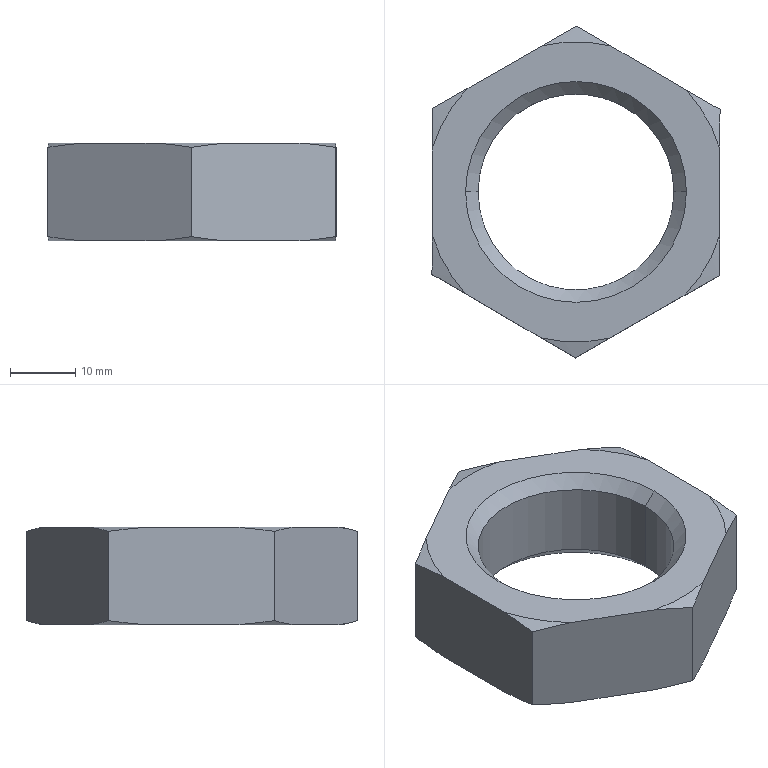Part | STEP file | GB/T6172.1-2000 hex thin nut grade A and B M30 | 1 solid | 26 faces | box 44.137 x 50.85 x 15 mm | volume 14200 mm3 | cone 16 | plane 8 | cylinder 2 | commonest cylinder face diameters 30 x2
STEP:
#1=CARTESIAN_POINT('',(-15.,0.,13.086));
#2=VERTEX_POINT('',#1);
#3=CARTESIAN_POINT('',(15.,0.,13.086));
#4=VERTEX_POINT('',#3);
#5=CARTESIAN_POINT('',(0.,0.,13.086));
#6=DIRECTION('',(0.,0.,1.));
#7=DIRECTION('',(1.,0.,0.));
#8=AXIS2_PLACEMENT_3D('',#5,#6,#7);
#9=CIRCLE('',#8,15.);
#10=EDGE_CURVE('',#2,#4,#9,.T.);
#11=ORIENTED_EDGE('',*,*,#10,.F.);
#12=CARTESIAN_POINT('',(-16.914,0.,15.));
#13=VERTEX_POINT('',#12);
#14=CARTESIAN_POINT('',(-15.,0.,13.086));
#15=DIRECTION('',(-0.7071,0.,0.7071));
#16=VECTOR('',#15,1000.);
#17=LINE('',#14,#16);
#18=EDGE_CURVE('',#2,#13,#17,.T.);
#19=ORIENTED_EDGE('',*,*,#18,.T.);
#20=CARTESIAN_POINT('',(16.914,0.,15.));
#21=VERTEX_POINT('',#20);
#22=CARTESIAN_POINT('',(0.,0.,15.));
#23=DIRECTION('',(0.,0.,-1.));
#24=DIRECTION('',(1.,0.,0.));
#25=AXIS2_PLACEMENT_3D('',#22,#23,#24);
#26=CIRCLE('',#25,16.914);
#27=EDGE_CURVE('',#21,#13,#26,.T.);
#28=ORIENTED_EDGE('',*,*,#27,.F.);
#29=CARTESIAN_POINT('',(15.,0.,13.086));
#30=DIRECTION('',(0.7071,0.,0.7071));
#31=VECTOR('',#30,1000.);
#32=LINE('',#29,#31);
#33=EDGE_CURVE('',#4,#21,#32,.T.);
#34=ORIENTED_EDGE('',*,*,#33,.F.);
#35=EDGE_LOOP('',(#11,#19,#28,#34));
#36=FACE_OUTER_BOUND('',#35,.T.);
#37=CARTESIAN_POINT('',(0.,0.,13.086));
#38=DIRECTION('',(0.,0.,1.));
#39=DIRECTION('',(1.,0.,0.));
#40=AXIS2_PLACEMENT_3D('',#37,#38,#39);
#41=CONICAL_SURFACE('',#40,15.,0.7854);
#42=ADVANCED_FACE('',(#36),#41,.F.);
#43=CARTESIAN_POINT('',(15.,0.,1.914));
#44=VERTEX_POINT('',#43);
#45=CARTESIAN_POINT('',(-15.,0.,1.914));
#46=VERTEX_POINT('',#45);
#47=CARTESIAN_POINT('',(0.,0.,1.914));
#48=DIRECTION('',(0.,0.,-1.));
#49=DIRECTION('',(1.,0.,0.));
#50=AXIS2_PLACEMENT_3D('',#47,#48,#49);
#51=CIRCLE('',#50,15.);
#52=EDGE_CURVE('',#44,#46,#51,.T.);
#53=ORIENTED_EDGE('',*,*,#52,.F.);
#54=CARTESIAN_POINT('',(16.914,0.,0.));
#55=VERTEX_POINT('',#54);
#56=CARTESIAN_POINT('',(16.914,0.,0.));
#57=DIRECTION('',(0.7071,0.,-0.7071));
#58=VECTOR('',#57,1000.);
#59=LINE('',#56,#58);
#60=EDGE_CURVE('',#44,#55,#59,.T.);
#61=ORIENTED_EDGE('',*,*,#60,.T.);
#62=CARTESIAN_POINT('',(-16.914,0.,0.));
#63=VERTEX_POINT('',#62);
#64=CARTESIAN_POINT('',(0.,0.,0.));
#65=DIRECTION('',(0.,0.,1.));
#66=DIRECTION('',(1.,0.,0.));
#67=AXIS2_PLACEMENT_3D('',#64,#65,#66);
#68=CIRCLE('',#67,16.914);
#69=EDGE_CURVE('',#63,#55,#68,.T.);
#70=ORIENTED_EDGE('',*,*,#69,.F.);
#71=CARTESIAN_POINT('',(-16.914,0.,0.));
#72=DIRECTION('',(-0.7071,0.,-0.7071));
#73=VECTOR('',#72,1000.);
#74=LINE('',#71,#73);
#75=EDGE_CURVE('',#46,#63,#74,.T.);
#76=ORIENTED_EDGE('',*,*,#75,.F.);
#77=EDGE_LOOP('',(#53,#61,#70,#76));
#78=FACE_OUTER_BOUND('',#77,.T.);
#79=CARTESIAN_POINT('',(0.,0.,0.));
#80=DIRECTION('',(0.,0.,-1.));
#81=DIRECTION('',(-1.,0.,0.));
#82=AXIS2_PLACEMENT_3D('',#79,#80,#81);
#83=CONICAL_SURFACE('',#82,16.914,0.7854);
#84=ADVANCED_FACE('',(#78),#83,.F.);
#85=ORIENTED_EDGE('',*,*,#10,.T.);
#86=CARTESIAN_POINT('',(15.,0.,15.));
#87=DIRECTION('',(0.,0.,-1.));
#88=VECTOR('',#87,1000.);
#89=LINE('',#86,#88);
#90=EDGE_CURVE('',#4,#44,#89,.T.);
#91=ORIENTED_EDGE('',*,*,#90,.T.);
#92=ORIENTED_EDGE('',*,*,#52,.T.);
#93=CARTESIAN_POINT('',(-15.,0.,15.));
#94=DIRECTION('',(0.,0.,-1.));
#95=VECTOR('',#94,1000.);
#96=LINE('',#93,#95);
#97=EDGE_CURVE('',#2,#46,#96,.T.);
#98=ORIENTED_EDGE('',*,*,#97,.F.);
#99=EDGE_LOOP('',(#85,#91,#92,#98));
#100=FACE_OUTER_BOUND('',#99,.T.);
#101=CARTESIAN_POINT('',(0.,0.,15.));
#102=DIRECTION('',(0.,0.,-1.));
#103=DIRECTION('',(-1.,0.,0.));
#104=AXIS2_PLACEMENT_3D('',#101,#102,#103);
#105=CYLINDRICAL_SURFACE('',#104,15.);
#106=ADVANCED_FACE('',(#100),#105,.F.);
#107=CARTESIAN_POINT('',(22.069,12.626,14.35));
#108=VERTEX_POINT('',#107);
#109=CARTESIAN_POINT('',(16.827,15.679,15.));
#110=VERTEX_POINT('',#109);
#111=CARTESIAN_POINT('',(22.069,12.626,14.35));
#112=CARTESIAN_POINT('',(20.327,13.641,14.62));
#113=CARTESIAN_POINT('',(18.58,14.658,14.843));
#114=CARTESIAN_POINT('',(16.827,15.679,15.));
#115=B_SPLINE_CURVE_WITH_KNOTS('',3,(#111,#112,#113,#114),.UNSPECIFIED.,.F.,.F.,(4,4),(0.0208,0.0269),.UNSPECIFIED.);
#116=EDGE_CURVE('',#108,#110,#115,.T.);
#117=ORIENTED_EDGE('',*,*,#116,.F.);
#118=CARTESIAN_POINT('',(22.069,12.626,0.6498));
#119=VERTEX_POINT('',#118);
#120=CARTESIAN_POINT('',(22.069,12.626,15.));
#121=DIRECTION('',(0.,0.,-1.));
#122=VECTOR('',#121,1000.);
#123=LINE('',#120,#122);
#124=EDGE_CURVE('',#108,#119,#123,.T.);
#125=ORIENTED_EDGE('',*,*,#124,.T.);
#126=CARTESIAN_POINT('',(16.827,15.679,0.));
#127=VERTEX_POINT('',#126);
#128=CARTESIAN_POINT('',(16.827,15.679,0.));
#129=CARTESIAN_POINT('',(17.704,15.169,0.07853));
#130=CARTESIAN_POINT('',(18.58,14.658,0.1736));
#131=CARTESIAN_POINT('',(20.327,13.64,0.3918));
#132=CARTESIAN_POINT('',(21.199,13.132,0.5149));
#133=CARTESIAN_POINT('',(22.069,12.626,0.6498));
#134=B_SPLINE_CURVE_WITH_KNOTS('',3,(#128,#129,#130,#131,#132,#133),.UNSPECIFIED.,.F.,.F.,(4,2,4),(0.04011,0.04311,0.04611),.UNSPECIFIED.);
#135=EDGE_CURVE('',#127,#119,#134,.T.);
#136=ORIENTED_EDGE('',*,*,#135,.F.);
#137=CARTESIAN_POINT('',(5.341,22.371,0.));
#138=VERTEX_POINT('',#137);
#139=CARTESIAN_POINT('',(22.069,12.626,0.));
#140=DIRECTION('',(-0.8641,0.5034,0.));
#141=VECTOR('',#140,1000.);
#142=LINE('',#139,#141);
#143=EDGE_CURVE('',#127,#138,#142,.T.);
#144=ORIENTED_EDGE('',*,*,#143,.T.);
#145=CARTESIAN_POINT('',(0.1,25.425,0.6498));
#146=VERTEX_POINT('',#145);
#147=CARTESIAN_POINT('',(0.1,25.425,0.6498));
#148=CARTESIAN_POINT('',(1.842,24.41,0.3797));
#149=CARTESIAN_POINT('',(3.589,23.392,0.1571));
#150=CARTESIAN_POINT('',(5.341,22.371,0.));
#151=B_SPLINE_CURVE_WITH_KNOTS('',3,(#147,#148,#149,#150),.UNSPECIFIED.,.F.,.F.,(4,4),(0.0208,0.0269),.UNSPECIFIED.);
#152=EDGE_CURVE('',#146,#138,#151,.T.);
#153=ORIENTED_EDGE('',*,*,#152,.F.);
#154=CARTESIAN_POINT('',(0.1,25.425,14.35));
#155=VERTEX_POINT('',#154);
#156=CARTESIAN_POINT('',(0.1,25.425,15.));
#157=DIRECTION('',(0.,0.,-1.));
#158=VECTOR('',#157,1000.);
#159=LINE('',#156,#158);
#160=EDGE_CURVE('',#155,#146,#159,.T.);
#161=ORIENTED_EDGE('',*,*,#160,.F.);
#162=CARTESIAN_POINT('',(5.341,22.371,15.));
#163=VERTEX_POINT('',#162);
#164=CARTESIAN_POINT('',(5.341,22.371,15.));
#165=CARTESIAN_POINT('',(4.465,22.882,14.921));
#166=CARTESIAN_POINT('',(3.588,23.393,14.826));
#167=CARTESIAN_POINT('',(1.841,24.41,14.608));
#168=CARTESIAN_POINT('',(0.9697,24.918,14.485));
#169=CARTESIAN_POINT('',(0.1,25.425,14.35));
#170=B_SPLINE_CURVE_WITH_KNOTS('',3,(#164,#165,#166,#167,#168,#169),.UNSPECIFIED.,.F.,.F.,(4,2,4),(0.04011,0.04311,0.04611),.UNSPECIFIED.);
#171=EDGE_CURVE('',#163,#155,#170,.T.);
#172=ORIENTED_EDGE('',*,*,#171,.F.);
#173=CARTESIAN_POINT('',(22.069,12.626,15.));
#174=DIRECTION('',(-0.8641,0.5034,0.));
#175=VECTOR('',#174,1000.);
#176=LINE('',#173,#175);
#177=EDGE_CURVE('',#110,#163,#176,.T.);
#178=ORIENTED_EDGE('',*,*,#177,.F.);
#179=EDGE_LOOP('',(#117,#125,#136,#144,#153,#161,#172,#178));
#180=FACE_OUTER_BOUND('',#179,.T.);
#181=CARTESIAN_POINT('',(22.069,12.626,15.));
#182=DIRECTION('',(-0.5034,-0.8641,0.));
#183=DIRECTION('',(0.8641,-0.5034,0.));
#184=AXIS2_PLACEMENT_3D('',#181,#182,#183);
#185=PLANE('',#184);
#186=ADVANCED_FACE('',(#180),#185,.F.);
#187=CARTESIAN_POINT('',(-5.165,22.413,15.));
#188=VERTEX_POINT('',#187);
#189=CARTESIAN_POINT('',(0.1,25.425,14.35));
#190=CARTESIAN_POINT('',(-1.65,24.424,14.62));
#191=CARTESIAN_POINT('',(-3.404,23.42,14.843));
#192=CARTESIAN_POINT('',(-5.165,22.413,15.));
#193=B_SPLINE_CURVE_WITH_KNOTS('',3,(#189,#190,#191,#192),.UNSPECIFIED.,.F.,.F.,(4,4),(0.0207,0.0268),.UNSPECIFIED.);
#194=EDGE_CURVE('',#155,#188,#193,.T.);
#195=ORIENTED_EDGE('',*,*,#194,.F.);
#196=ORIENTED_EDGE('',*,*,#160,.T.);
#197=CARTESIAN_POINT('',(-5.165,22.413,0.));
#198=VERTEX_POINT('',#197);
#199=CARTESIAN_POINT('',(-5.165,22.413,0.));
#200=CARTESIAN_POINT('',(-4.285,22.916,0.07852));
#201=CARTESIAN_POINT('',(-3.404,23.42,0.1736));
#202=CARTESIAN_POINT('',(-1.649,24.424,0.3918));
#203=CARTESIAN_POINT('',(-0.7736,24.925,0.5149));
#204=CARTESIAN_POINT('',(0.1,25.425,0.6498));
#205=B_SPLINE_CURVE_WITH_KNOTS('',3,(#199,#200,#201,#202,#203,#204),.UNSPECIFIED.,.F.,.F.,(4,2,4),(0.04002,0.04302,0.04602),.UNSPECIFIED.);
#206=EDGE_CURVE('',#198,#146,#205,.T.);
#207=ORIENTED_EDGE('',*,*,#206,.F.);
#208=CARTESIAN_POINT('',(-16.703,15.811,0.));
#209=VERTEX_POINT('',#208);
#210=CARTESIAN_POINT('',(0.1,25.425,0.));
#211=DIRECTION('',(-0.868,-0.4966,0.));
#212=VECTOR('',#211,1000.);
#213=LINE('',#210,#212);
#214=EDGE_CURVE('',#198,#209,#213,.T.);
#215=ORIENTED_EDGE('',*,*,#214,.T.);
#216=CARTESIAN_POINT('',(-21.969,12.799,0.6498));
#217=VERTEX_POINT('',#216);
#218=CARTESIAN_POINT('',(-21.969,12.799,0.6498));
#219=CARTESIAN_POINT('',(-20.219,13.8,0.3797));
#220=CARTESIAN_POINT('',(-18.464,14.804,0.1571));
#221=CARTESIAN_POINT('',(-16.703,15.811,0.));
#222=B_SPLINE_CURVE_WITH_KNOTS('',3,(#218,#219,#220,#221),.UNSPECIFIED.,.F.,.F.,(4,4),(0.0207,0.0268),.UNSPECIFIED.);
#223=EDGE_CURVE('',#217,#209,#222,.T.);
#224=ORIENTED_EDGE('',*,*,#223,.F.);
#225=CARTESIAN_POINT('',(-21.969,12.799,14.35));
#226=VERTEX_POINT('',#225);
#227=CARTESIAN_POINT('',(-21.969,12.799,15.));
#228=DIRECTION('',(0.,0.,-1.));
#229=VECTOR('',#228,1000.);
#230=LINE('',#227,#229);
#231=EDGE_CURVE('',#226,#217,#230,.T.);
#232=ORIENTED_EDGE('',*,*,#231,.F.);
#233=CARTESIAN_POINT('',(-16.703,15.811,15.));
#234=VERTEX_POINT('',#233);
#235=CARTESIAN_POINT('',(-16.703,15.811,15.));
#236=CARTESIAN_POINT('',(-17.584,15.308,14.921));
#237=CARTESIAN_POINT('',(-18.464,14.804,14.826));
#238=CARTESIAN_POINT('',(-20.219,13.8,14.608));
#239=CARTESIAN_POINT('',(-21.095,13.299,14.485));
#240=CARTESIAN_POINT('',(-21.969,12.799,14.35));
#241=B_SPLINE_CURVE_WITH_KNOTS('',3,(#235,#236,#237,#238,#239,#240),.UNSPECIFIED.,.F.,.F.,(4,2,4),(0.04002,0.04302,0.04602),.UNSPECIFIED.);
#242=EDGE_CURVE('',#234,#226,#241,.T.);
#243=ORIENTED_EDGE('',*,*,#242,.F.);
#244=CARTESIAN_POINT('',(0.1,25.425,15.));
#245=DIRECTION('',(-0.868,-0.4966,0.));
#246=VECTOR('',#245,1000.);
#247=LINE('',#244,#246);
#248=EDGE_CURVE('',#188,#234,#247,.T.);
#249=ORIENTED_EDGE('',*,*,#248,.F.);
#250=EDGE_LOOP('',(#195,#196,#207,#215,#224,#232,#243,#249));
#251=FACE_OUTER_BOUND('',#250,.T.);
#252=CARTESIAN_POINT('',(0.1,25.425,15.));
#253=DIRECTION('',(0.4966,-0.868,0.));
#254=DIRECTION('',(0.868,0.4966,0.));
#255=AXIS2_PLACEMENT_3D('',#252,#253,#254);
#256=PLANE('',#255);
#257=ADVANCED_FACE('',(#251),#256,.F.);
#258=CARTESIAN_POINT('',(-21.992,6.733,15.));
#259=VERTEX_POINT('',#258);
#260=CARTESIAN_POINT('',(-21.969,12.799,14.35));
#261=CARTESIAN_POINT('',(-21.976,10.782,14.62));
#262=CARTESIAN_POINT('',(-21.984,8.761,14.843));
#263=CARTESIAN_POINT('',(-21.992,6.733,15.));
#264=B_SPLINE_CURVE_WITH_KNOTS('',3,(#260,#261,#262,#263),.UNSPECIFIED.,.F.,.F.,(4,4),(0.01795,0.02405),.UNSPECIFIED.);
#265=EDGE_CURVE('',#226,#259,#264,.T.);
#266=ORIENTED_EDGE('',*,*,#265,.F.);
#267=ORIENTED_EDGE('',*,*,#231,.T.);
#268=CARTESIAN_POINT('',(-21.992,6.733,0.));
#269=VERTEX_POINT('',#268);
#270=CARTESIAN_POINT('',(-21.992,6.733,0.));
#271=CARTESIAN_POINT('',(-21.988,7.746,0.07843));
#272=CARTESIAN_POINT('',(-21.984,8.761,0.1735));
#273=CARTESIAN_POINT('',(-21.976,10.783,0.3917));
#274=CARTESIAN_POINT('',(-21.972,11.792,0.5149));
#275=CARTESIAN_POINT('',(-21.969,12.799,0.6498));
#276=B_SPLINE_CURVE_WITH_KNOTS('',3,(#270,#271,#272,#273,#274,#275),.UNSPECIFIED.,.F.,.F.,(4,2,4),(0.03728,0.04028,0.04328),.UNSPECIFIED.);
#277=EDGE_CURVE('',#269,#217,#276,.T.);
#278=ORIENTED_EDGE('',*,*,#277,.F.);
#279=CARTESIAN_POINT('',(-22.045,-6.56,0.));
#280=VERTEX_POINT('',#279);
#281=CARTESIAN_POINT('',(-21.969,12.799,0.));
#282=DIRECTION('',(-0.003934,-1.,0.));
#283=VECTOR('',#282,1000.);
#284=LINE('',#281,#283);
#285=EDGE_CURVE('',#269,#280,#284,.T.);
#286=ORIENTED_EDGE('',*,*,#285,.T.);
#287=CARTESIAN_POINT('',(-22.069,-12.626,0.6498));
#288=VERTEX_POINT('',#287);
#289=CARTESIAN_POINT('',(-22.069,-12.626,0.6498));
#290=CARTESIAN_POINT('',(-22.061,-10.609,0.3796));
#291=CARTESIAN_POINT('',(-22.053,-8.588,0.157));
#292=CARTESIAN_POINT('',(-22.045,-6.56,0.));
#293=B_SPLINE_CURVE_WITH_KNOTS('',3,(#289,#290,#291,#292),.UNSPECIFIED.,.F.,.F.,(4,4),(0.01795,0.02405),.UNSPECIFIED.);
#294=EDGE_CURVE('',#288,#280,#293,.T.);
#295=ORIENTED_EDGE('',*,*,#294,.F.);
#296=CARTESIAN_POINT('',(-22.069,-12.626,14.35));
#297=VERTEX_POINT('',#296);
#298=CARTESIAN_POINT('',(-22.069,-12.626,15.));
#299=DIRECTION('',(0.,0.,-1.));
#300=VECTOR('',#299,1000.);
#301=LINE('',#298,#300);
#302=EDGE_CURVE('',#297,#288,#301,.T.);
#303=ORIENTED_EDGE('',*,*,#302,.F.);
#304=CARTESIAN_POINT('',(-22.045,-6.56,15.));
#305=VERTEX_POINT('',#304);
#306=CARTESIAN_POINT('',(-22.045,-6.56,15.));
#307=CARTESIAN_POINT('',(-22.049,-7.573,14.922));
#308=CARTESIAN_POINT('',(-22.053,-8.588,14.826));
#309=CARTESIAN_POINT('',(-22.061,-10.61,14.608));
#310=CARTESIAN_POINT('',(-22.065,-11.619,14.485));
#311=CARTESIAN_POINT('',(-22.069,-12.626,14.35));
#312=B_SPLINE_CURVE_WITH_KNOTS('',3,(#306,#307,#308,#309,#310,#311),.UNSPECIFIED.,.F.,.F.,(4,2,4),(0.03728,0.04028,0.04328),.UNSPECIFIED.);
#313=EDGE_CURVE('',#305,#297,#312,.T.);
#314=ORIENTED_EDGE('',*,*,#313,.F.);
#315=CARTESIAN_POINT('',(-21.969,12.799,15.));
#316=DIRECTION('',(-0.003934,-1.,0.));
#317=VECTOR('',#316,1000.);
#318=LINE('',#315,#317);
#319=EDGE_CURVE('',#259,#305,#318,.T.);
#320=ORIENTED_EDGE('',*,*,#319,.F.);
#321=EDGE_LOOP('',(#266,#267,#278,#286,#295,#303,#314,#320));
#322=FACE_OUTER_BOUND('',#321,.T.);
#323=CARTESIAN_POINT('',(-21.969,12.799,15.));
#324=DIRECTION('',(1.,-0.003934,0.));
#325=DIRECTION('',(0.003934,1.,0.));
#326=AXIS2_PLACEMENT_3D('',#323,#324,#325);
#327=PLANE('',#326);
#328=ADVANCED_FACE('',(#322),#327,.F.);
#329=CARTESIAN_POINT('',(-16.827,-15.679,15.));
#330=VERTEX_POINT('',#329);
#331=CARTESIAN_POINT('',(-22.069,-12.626,14.35));
#332=CARTESIAN_POINT('',(-20.327,-13.641,14.62));
#333=CARTESIAN_POINT('',(-18.58,-14.658,14.843));
#334=CARTESIAN_POINT('',(-16.827,-15.679,15.));
#335=B_SPLINE_CURVE_WITH_KNOTS('',3,(#331,#332,#333,#334),.UNSPECIFIED.,.F.,.F.,(4,4),(0.0208,0.0269),.UNSPECIFIED.);
#336=EDGE_CURVE('',#297,#330,#335,.T.);
#337=ORIENTED_EDGE('',*,*,#336,.F.);
#338=ORIENTED_EDGE('',*,*,#302,.T.);
#339=CARTESIAN_POINT('',(-16.827,-15.679,0.));
#340=VERTEX_POINT('',#339);
#341=CARTESIAN_POINT('',(-16.827,-15.679,0.));
#342=CARTESIAN_POINT('',(-17.704,-15.169,0.07853));
#343=CARTESIAN_POINT('',(-18.58,-14.658,0.1736));
#344=CARTESIAN_POINT('',(-20.327,-13.64,0.3918));
#345=CARTESIAN_POINT('',(-21.199,-13.132,0.5149));
#346=CARTESIAN_POINT('',(-22.069,-12.626,0.6498));
#347=B_SPLINE_CURVE_WITH_KNOTS('',3,(#341,#342,#343,#344,#345,#346),.UNSPECIFIED.,.F.,.F.,(4,2,4),(0.04011,0.04311,0.04611),.UNSPECIFIED.);
#348=EDGE_CURVE('',#340,#288,#347,.T.);
#349=ORIENTED_EDGE('',*,*,#348,.F.);
#350=CARTESIAN_POINT('',(-5.341,-22.371,0.));
#351=VERTEX_POINT('',#350);
#352=CARTESIAN_POINT('',(-22.069,-12.626,0.));
#353=DIRECTION('',(0.8641,-0.5034,0.));
#354=VECTOR('',#353,1000.);
#355=LINE('',#352,#354);
#356=EDGE_CURVE('',#340,#351,#355,.T.);
#357=ORIENTED_EDGE('',*,*,#356,.T.);
#358=CARTESIAN_POINT('',(-0.1,-25.425,0.6498));
#359=VERTEX_POINT('',#358);
#360=CARTESIAN_POINT('',(-0.1,-25.425,0.6498));
#361=CARTESIAN_POINT('',(-1.842,-24.41,0.3797));
#362=CARTESIAN_POINT('',(-3.589,-23.392,0.1571));
#363=CARTESIAN_POINT('',(-5.341,-22.371,0.));
#364=B_SPLINE_CURVE_WITH_KNOTS('',3,(#360,#361,#362,#363),.UNSPECIFIED.,.F.,.F.,(4,4),(0.0208,0.0269),.UNSPECIFIED.);
#365=EDGE_CURVE('',#359,#351,#364,.T.);
#366=ORIENTED_EDGE('',*,*,#365,.F.);
#367=CARTESIAN_POINT('',(-0.1,-25.425,14.35));
#368=VERTEX_POINT('',#367);
#369=CARTESIAN_POINT('',(-0.1,-25.425,15.));
#370=DIRECTION('',(0.,0.,-1.));
#371=VECTOR('',#370,1000.);
#372=LINE('',#369,#371);
#373=EDGE_CURVE('',#368,#359,#372,.T.);
#374=ORIENTED_EDGE('',*,*,#373,.F.);
#375=CARTESIAN_POINT('',(-5.341,-22.371,15.));
#376=VERTEX_POINT('',#375);
#377=CARTESIAN_POINT('',(-5.341,-22.371,15.));
#378=CARTESIAN_POINT('',(-4.465,-22.882,14.921));
#379=CARTESIAN_POINT('',(-3.588,-23.393,14.826));
#380=CARTESIAN_POINT('',(-1.841,-24.41,14.608));
#381=CARTESIAN_POINT('',(-0.9697,-24.918,14.485));
#382=CARTESIAN_POINT('',(-0.1,-25.425,14.35));
#383=B_SPLINE_CURVE_WITH_KNOTS('',3,(#377,#378,#379,#380,#381,#382),.UNSPECIFIED.,.F.,.F.,(4,2,4),(0.04011,0.04311,0.04611),.UNSPECIFIED.);
#384=EDGE_CURVE('',#376,#368,#383,.T.);
#385=ORIENTED_EDGE('',*,*,#384,.F.);
#386=CARTESIAN_POINT('',(-22.069,-12.626,15.));
#387=DIRECTION('',(0.8641,-0.5034,0.));
#388=VECTOR('',#387,1000.);
#389=LINE('',#386,#388);
#390=EDGE_CURVE('',#330,#376,#389,.T.);
#391=ORIENTED_EDGE('',*,*,#390,.F.);
#392=EDGE_LOOP('',(#337,#338,#349,#357,#366,#374,#385,#391));
#393=FACE_OUTER_BOUND('',#392,.T.);
#394=CARTESIAN_POINT('',(-22.069,-12.626,15.));
#395=DIRECTION('',(0.5034,0.8641,0.));
#396=DIRECTION('',(-0.8641,0.5034,0.));
#397=AXIS2_PLACEMENT_3D('',#394,#395,#396);
#398=PLANE('',#397);
#399=ADVANCED_FACE('',(#393),#398,.F.);
#400=CARTESIAN_POINT('',(5.165,-22.413,15.));
#401=VERTEX_POINT('',#400);
#402=CARTESIAN_POINT('',(-0.1,-25.425,14.35));
#403=CARTESIAN_POINT('',(1.65,-24.424,14.62));
#404=CARTESIAN_POINT('',(3.404,-23.42,14.843));
#405=CARTESIAN_POINT('',(5.165,-22.413,15.));
#406=B_SPLINE_CURVE_WITH_KNOTS('',3,(#402,#403,#404,#405),.UNSPECIFIED.,.F.,.F.,(4,4),(0.0207,0.0268),.UNSPECIFIED.);
#407=EDGE_CURVE('',#368,#401,#406,.T.);
#408=ORIENTED_EDGE('',*,*,#407,.F.);
#409=ORIENTED_EDGE('',*,*,#373,.T.);
#410=CARTESIAN_POINT('',(5.165,-22.413,0.));
#411=VERTEX_POINT('',#410);
#412=CARTESIAN_POINT('',(5.165,-22.413,0.));
#413=CARTESIAN_POINT('',(4.285,-22.916,0.07852));
#414=CARTESIAN_POINT('',(3.404,-23.42,0.1736));
#415=CARTESIAN_POINT('',(1.649,-24.424,0.3918));
#416=CARTESIAN_POINT('',(0.7736,-24.925,0.5149));
#417=CARTESIAN_POINT('',(-0.1,-25.425,0.6498));
#418=B_SPLINE_CURVE_WITH_KNOTS('',3,(#412,#413,#414,#415,#416,#417),.UNSPECIFIED.,.F.,.F.,(4,2,4),(0.04002,0.04302,0.04602),.UNSPECIFIED.);
#419=EDGE_CURVE('',#411,#359,#418,.T.);
#420=ORIENTED_EDGE('',*,*,#419,.F.);
#421=CARTESIAN_POINT('',(16.703,-15.811,0.));
#422=VERTEX_POINT('',#421);
#423=CARTESIAN_POINT('',(-0.1,-25.425,0.));
#424=DIRECTION('',(0.868,0.4966,0.));
#425=VECTOR('',#424,1000.);
#426=LINE('',#423,#425);
#427=EDGE_CURVE('',#411,#422,#426,.T.);
#428=ORIENTED_EDGE('',*,*,#427,.T.);
#429=CARTESIAN_POINT('',(21.969,-12.799,0.6498));
#430=VERTEX_POINT('',#429);
#431=CARTESIAN_POINT('',(21.969,-12.799,0.6498));
#432=CARTESIAN_POINT('',(20.219,-13.8,0.3797));
#433=CARTESIAN_POINT('',(18.464,-14.804,0.1571));
#434=CARTESIAN_POINT('',(16.703,-15.811,0.));
#435=B_SPLINE_CURVE_WITH_KNOTS('',3,(#431,#432,#433,#434),.UNSPECIFIED.,.F.,.F.,(4,4),(0.0207,0.0268),.UNSPECIFIED.);
#436=EDGE_CURVE('',#430,#422,#435,.T.);
#437=ORIENTED_EDGE('',*,*,#436,.F.);
#438=CARTESIAN_POINT('',(21.969,-12.799,14.35));
#439=VERTEX_POINT('',#438);
#440=CARTESIAN_POINT('',(21.969,-12.799,15.));
#441=DIRECTION('',(0.,0.,-1.));
#442=VECTOR('',#441,1000.);
#443=LINE('',#440,#442);
#444=EDGE_CURVE('',#439,#430,#443,.T.);
#445=ORIENTED_EDGE('',*,*,#444,.F.);
#446=CARTESIAN_POINT('',(16.703,-15.811,15.));
#447=VERTEX_POINT('',#446);
#448=CARTESIAN_POINT('',(16.703,-15.811,15.));
#449=CARTESIAN_POINT('',(17.584,-15.308,14.921));
#450=CARTESIAN_POINT('',(18.464,-14.804,14.826));
#451=CARTESIAN_POINT('',(20.219,-13.8,14.608));
#452=CARTESIAN_POINT('',(21.095,-13.299,14.485));
#453=CARTESIAN_POINT('',(21.969,-12.799,14.35));
#454=B_SPLINE_CURVE_WITH_KNOTS('',3,(#448,#449,#450,#451,#452,#453),.UNSPECIFIED.,.F.,.F.,(4,2,4),(0.04002,0.04302,0.04602),.UNSPECIFIED.);
#455=EDGE_CURVE('',#447,#439,#454,.T.);
#456=ORIENTED_EDGE('',*,*,#455,.F.);
#457=CARTESIAN_POINT('',(-0.1,-25.425,15.));
#458=DIRECTION('',(0.868,0.4966,0.));
#459=VECTOR('',#458,1000.);
#460=LINE('',#457,#459);
#461=EDGE_CURVE('',#401,#447,#460,.T.);
#462=ORIENTED_EDGE('',*,*,#461,.F.);
#463=EDGE_LOOP('',(#408,#409,#420,#428,#437,#445,#456,#462));
#464=FACE_OUTER_BOUND('',#463,.T.);
#465=CARTESIAN_POINT('',(-0.1,-25.425,15.));
#466=DIRECTION('',(-0.4966,0.868,0.));
#467=DIRECTION('',(-0.868,-0.4966,0.));
#468=AXIS2_PLACEMENT_3D('',#465,#466,#467);
#469=PLANE('',#468);
#470=ADVANCED_FACE('',(#464),#469,.F.);
#471=CARTESIAN_POINT('',(21.992,-6.733,15.));
#472=VERTEX_POINT('',#471);
#473=CARTESIAN_POINT('',(21.969,-12.799,14.35));
#474=CARTESIAN_POINT('',(21.976,-10.782,14.62));
#475=CARTESIAN_POINT('',(21.984,-8.761,14.843));
#476=CARTESIAN_POINT('',(21.992,-6.733,15.));
#477=B_SPLINE_CURVE_WITH_KNOTS('',3,(#473,#474,#475,#476),.UNSPECIFIED.,.F.,.F.,(4,4),(0.01795,0.02405),.UNSPECIFIED.);
#478=EDGE_CURVE('',#439,#472,#477,.T.);
#479=ORIENTED_EDGE('',*,*,#478,.F.);
#480=ORIENTED_EDGE('',*,*,#444,.T.);
#481=CARTESIAN_POINT('',(21.992,-6.733,0.));
#482=VERTEX_POINT('',#481);
#483=CARTESIAN_POINT('',(21.992,-6.733,0.));
#484=CARTESIAN_POINT('',(21.988,-7.746,0.07843));
#485=CARTESIAN_POINT('',(21.984,-8.761,0.1735));
#486=CARTESIAN_POINT('',(21.976,-10.783,0.3917));
#487=CARTESIAN_POINT('',(21.972,-11.792,0.5149));
#488=CARTESIAN_POINT('',(21.969,-12.799,0.6498));
#489=B_SPLINE_CURVE_WITH_KNOTS('',3,(#483,#484,#485,#486,#487,#488),.UNSPECIFIED.,.F.,.F.,(4,2,4),(0.03728,0.04028,0.04328),.UNSPECIFIED.);
#490=EDGE_CURVE('',#482,#430,#489,.T.);
#491=ORIENTED_EDGE('',*,*,#490,.F.);
#492=CARTESIAN_POINT('',(22.045,6.56,0.));
#493=VERTEX_POINT('',#492);
#494=CARTESIAN_POINT('',(21.969,-12.799,0.));
#495=DIRECTION('',(0.003934,1.,0.));
#496=VECTOR('',#495,1000.);
#497=LINE('',#494,#496);
#498=EDGE_CURVE('',#482,#493,#497,.T.);
#499=ORIENTED_EDGE('',*,*,#498,.T.);
#500=CARTESIAN_POINT('',(22.069,12.626,0.6498));
#501=CARTESIAN_POINT('',(22.061,10.609,0.3796));
#502=CARTESIAN_POINT('',(22.053,8.588,0.157));
#503=CARTESIAN_POINT('',(22.045,6.56,0.));
#504=B_SPLINE_CURVE_WITH_KNOTS('',3,(#500,#501,#502,#503),.UNSPECIFIED.,.F.,.F.,(4,4),(0.01795,0.02405),.UNSPECIFIED.);
#505=EDGE_CURVE('',#119,#493,#504,.T.);
#506=ORIENTED_EDGE('',*,*,#505,.F.);
#507=ORIENTED_EDGE('',*,*,#124,.F.);
#508=CARTESIAN_POINT('',(22.045,6.56,15.));
#509=VERTEX_POINT('',#508);
#510=CARTESIAN_POINT('',(22.045,6.56,15.));
#511=CARTESIAN_POINT('',(22.049,7.573,14.922));
#512=CARTESIAN_POINT('',(22.053,8.588,14.826));
#513=CARTESIAN_POINT('',(22.061,10.61,14.608));
#514=CARTESIAN_POINT('',(22.065,11.619,14.485));
#515=CARTESIAN_POINT('',(22.069,12.626,14.35));
#516=B_SPLINE_CURVE_WITH_KNOTS('',3,(#510,#511,#512,#513,#514,#515),.UNSPECIFIED.,.F.,.F.,(4,2,4),(0.03728,0.04028,0.04328),.UNSPECIFIED.);
#517=EDGE_CURVE('',#509,#108,#516,.T.);
#518=ORIENTED_EDGE('',*,*,#517,.F.);
#519=CARTESIAN_POINT('',(21.969,-12.799,15.));
#520=DIRECTION('',(0.003934,1.,0.));
#521=VECTOR('',#520,1000.);
#522=LINE('',#519,#521);
#523=EDGE_CURVE('',#472,#509,#522,.T.);
#524=ORIENTED_EDGE('',*,*,#523,.F.);
#525=EDGE_LOOP('',(#479,#480,#491,#499,#506,#507,#518,#524));
#526=FACE_OUTER_BOUND('',#525,.T.);
#527=CARTESIAN_POINT('',(21.969,-12.799,15.));
#528=DIRECTION('',(-1.,0.003934,0.));
#529=DIRECTION('',(-0.003934,-1.,0.));
#530=AXIS2_PLACEMENT_3D('',#527,#528,#529);
#531=PLANE('',#530);
#532=ADVANCED_FACE('',(#526),#531,.F.);
#533=ORIENTED_EDGE('',*,*,#27,.T.);
#534=CARTESIAN_POINT('',(0.,0.,15.));
#535=DIRECTION('',(0.,0.,-1.));
#536=DIRECTION('',(1.,0.,0.));
#537=AXIS2_PLACEMENT_3D('',#534,#535,#536);
#538=CIRCLE('',#537,16.914);
#539=EDGE_CURVE('',#13,#21,#538,.T.);
#540=ORIENTED_EDGE('',*,*,#539,.T.);
#541=EDGE_LOOP('',(#533,#540));
#542=FACE_BOUND('',#541,.T.);
#543=ORIENTED_EDGE('',*,*,#523,.T.);
#544=CARTESIAN_POINT('',(0.,0.,15.));
#545=DIRECTION('',(0.,0.,1.));
#546=DIRECTION('',(1.,0.,0.));
#547=AXIS2_PLACEMENT_3D('',#544,#545,#546);
#548=CIRCLE('',#547,23.);
#549=EDGE_CURVE('',#509,#110,#548,.T.);
#550=ORIENTED_EDGE('',*,*,#549,.T.);
#551=ORIENTED_EDGE('',*,*,#177,.T.);
#552=CARTESIAN_POINT('',(0.,0.,15.));
#553=DIRECTION('',(0.,0.,1.));
#554=DIRECTION('',(1.,0.,0.));
#555=AXIS2_PLACEMENT_3D('',#552,#553,#554);
#556=CIRCLE('',#555,23.);
#557=EDGE_CURVE('',#163,#188,#556,.T.);
#558=ORIENTED_EDGE('',*,*,#557,.T.);
#559=ORIENTED_EDGE('',*,*,#248,.T.);
#560=CARTESIAN_POINT('',(0.,0.,15.));
#561=DIRECTION('',(0.,0.,1.));
#562=DIRECTION('',(1.,0.,0.));
#563=AXIS2_PLACEMENT_3D('',#560,#561,#562);
#564=CIRCLE('',#563,23.);
#565=EDGE_CURVE('',#234,#259,#564,.T.);
#566=ORIENTED_EDGE('',*,*,#565,.T.);
#567=ORIENTED_EDGE('',*,*,#319,.T.);
#568=CARTESIAN_POINT('',(0.,0.,15.));
#569=DIRECTION('',(0.,0.,1.));
#570=DIRECTION('',(1.,0.,0.));
#571=AXIS2_PLACEMENT_3D('',#568,#569,#570);
#572=CIRCLE('',#571,23.);
#573=EDGE_CURVE('',#305,#330,#572,.T.);
#574=ORIENTED_EDGE('',*,*,#573,.T.);
#575=ORIENTED_EDGE('',*,*,#390,.T.);
#576=CARTESIAN_POINT('',(0.,0.,15.));
#577=DIRECTION('',(0.,0.,1.));
#578=DIRECTION('',(1.,0.,0.));
#579=AXIS2_PLACEMENT_3D('',#576,#577,#578);
#580=CIRCLE('',#579,23.);
#581=EDGE_CURVE('',#376,#401,#580,.T.);
#582=ORIENTED_EDGE('',*,*,#581,.T.);
#583=ORIENTED_EDGE('',*,*,#461,.T.);
#584=CARTESIAN_POINT('',(0.,0.,15.));
#585=DIRECTION('',(0.,0.,1.));
#586=DIRECTION('',(1.,0.,0.));
#587=AXIS2_PLACEMENT_3D('',#584,#585,#586);
#588=CIRCLE('',#587,23.);
#589=EDGE_CURVE('',#447,#472,#588,.T.);
#590=ORIENTED_EDGE('',*,*,#589,.T.);
#591=EDGE_LOOP('',(#543,#550,#551,#558,#559,#566,#567,#574,#575,#582,#583,#590));
#592=FACE_OUTER_BOUND('',#591,.T.);
#593=CARTESIAN_POINT('',(0.1,25.425,15.));
#594=DIRECTION('',(0.,0.,1.));
#595=DIRECTION('',(1.,0.,0.));
#596=AXIS2_PLACEMENT_3D('',#593,#594,#595);
#597=PLANE('',#596);
#598=ADVANCED_FACE('',(#542,#592),#597,.T.);
#599=ORIENTED_EDGE('',*,*,#69,.T.);
#600=CARTESIAN_POINT('',(0.,0.,0.));
#601=DIRECTION('',(0.,0.,1.));
#602=DIRECTION('',(1.,0.,0.));
#603=AXIS2_PLACEMENT_3D('',#600,#601,#602);
#604=CIRCLE('',#603,16.914);
#605=EDGE_CURVE('',#55,#63,#604,.T.);
#606=ORIENTED_EDGE('',*,*,#605,.T.);
#607=EDGE_LOOP('',(#599,#606));
#608=FACE_BOUND('',#607,.T.);
#609=CARTESIAN_POINT('',(0.,0.,0.));
#610=DIRECTION('',(0.,0.,-1.));
#611=DIRECTION('',(-1.,0.,0.));
#612=AXIS2_PLACEMENT_3D('',#609,#610,#611);
#613=CIRCLE('',#612,23.);
#614=EDGE_CURVE('',#127,#493,#613,.T.);
#615=ORIENTED_EDGE('',*,*,#614,.T.);
#616=ORIENTED_EDGE('',*,*,#498,.F.);
#617=CARTESIAN_POINT('',(0.,0.,0.));
#618=DIRECTION('',(0.,0.,-1.));
#619=DIRECTION('',(-1.,0.,0.));
#620=AXIS2_PLACEMENT_3D('',#617,#618,#619);
#621=CIRCLE('',#620,23.);
#622=EDGE_CURVE('',#482,#422,#621,.T.);
#623=ORIENTED_EDGE('',*,*,#622,.T.);
#624=ORIENTED_EDGE('',*,*,#427,.F.);
#625=CARTESIAN_POINT('',(0.,0.,0.));
#626=DIRECTION('',(0.,0.,-1.));
#627=DIRECTION('',(-1.,0.,0.));
#628=AXIS2_PLACEMENT_3D('',#625,#626,#627);
#629=CIRCLE('',#628,23.);
#630=EDGE_CURVE('',#411,#351,#629,.T.);
#631=ORIENTED_EDGE('',*,*,#630,.T.);
#632=ORIENTED_EDGE('',*,*,#356,.F.);
#633=CARTESIAN_POINT('',(0.,0.,0.));
#634=DIRECTION('',(0.,0.,-1.));
#635=DIRECTION('',(-1.,0.,0.));
#636=AXIS2_PLACEMENT_3D('',#633,#634,#635);
#637=CIRCLE('',#636,23.);
#638=EDGE_CURVE('',#340,#280,#637,.T.);
#639=ORIENTED_EDGE('',*,*,#638,.T.);
#640=ORIENTED_EDGE('',*,*,#285,.F.);
#641=CARTESIAN_POINT('',(0.,0.,0.));
#642=DIRECTION('',(0.,0.,-1.));
#643=DIRECTION('',(-1.,0.,0.));
#644=AXIS2_PLACEMENT_3D('',#641,#642,#643);
#645=CIRCLE('',#644,23.);
#646=EDGE_CURVE('',#269,#209,#645,.T.);
#647=ORIENTED_EDGE('',*,*,#646,.T.);
#648=ORIENTED_EDGE('',*,*,#214,.F.);
#649=CARTESIAN_POINT('',(0.,0.,0.));
#650=DIRECTION('',(0.,0.,-1.));
#651=DIRECTION('',(-1.,0.,0.));
#652=AXIS2_PLACEMENT_3D('',#649,#650,#651);
#653=CIRCLE('',#652,23.);
#654=EDGE_CURVE('',#198,#138,#653,.T.);
#655=ORIENTED_EDGE('',*,*,#654,.T.);
#656=ORIENTED_EDGE('',*,*,#143,.F.);
#657=EDGE_LOOP('',(#615,#616,#623,#624,#631,#632,#639,#640,#647,#648,#655,#656));
#658=FACE_OUTER_BOUND('',#657,.T.);
#659=CARTESIAN_POINT('',(0.1,25.425,0.));
#660=DIRECTION('',(0.,0.,1.));
#661=DIRECTION('',(1.,0.,0.));
#662=AXIS2_PLACEMENT_3D('',#659,#660,#661);
#663=PLANE('',#662);
#664=ADVANCED_FACE('',(#608,#658),#663,.F.);
#665=ORIENTED_EDGE('',*,*,#90,.F.);
#666=CARTESIAN_POINT('',(0.,0.,13.086));
#667=DIRECTION('',(0.,0.,1.));
#668=DIRECTION('',(1.,0.,0.));
#669=AXIS2_PLACEMENT_3D('',#666,#667,#668);
#670=CIRCLE('',#669,15.);
#671=EDGE_CURVE('',#4,#2,#670,.T.);
#672=ORIENTED_EDGE('',*,*,#671,.T.);
#673=ORIENTED_EDGE('',*,*,#97,.T.);
#674=CARTESIAN_POINT('',(0.,0.,1.914));
#675=DIRECTION('',(0.,0.,-1.));
#676=DIRECTION('',(1.,0.,0.));
#677=AXIS2_PLACEMENT_3D('',#674,#675,#676);
#678=CIRCLE('',#677,15.);
#679=EDGE_CURVE('',#46,#44,#678,.T.);
#680=ORIENTED_EDGE('',*,*,#679,.T.);
#681=EDGE_LOOP('',(#665,#672,#673,#680));
#682=FACE_OUTER_BOUND('',#681,.T.);
#683=CARTESIAN_POINT('',(0.,0.,15.));
#684=DIRECTION('',(0.,0.,-1.));
#685=DIRECTION('',(-1.,0.,0.));
#686=AXIS2_PLACEMENT_3D('',#683,#684,#685);
#687=CYLINDRICAL_SURFACE('',#686,15.);
#688=ADVANCED_FACE('',(#682),#687,.F.);
#689=ORIENTED_EDGE('',*,*,#436,.T.);
#690=ORIENTED_EDGE('',*,*,#622,.F.);
#691=ORIENTED_EDGE('',*,*,#490,.T.);
#692=EDGE_LOOP('',(#689,#690,#691));
#693=FACE_OUTER_BOUND('',#692,.T.);
#694=CARTESIAN_POINT('',(0.,0.,0.));
#695=DIRECTION('',(0.,0.,1.));
#696=DIRECTION('',(-1.,0.,0.));
#697=AXIS2_PLACEMENT_3D('',#694,#695,#696);
#698=CONICAL_SURFACE('',#697,23.,1.309);
#699=ADVANCED_FACE('',(#693),#698,.T.);
#700=ORIENTED_EDGE('',*,*,#135,.T.);
#701=ORIENTED_EDGE('',*,*,#505,.T.);
#702=ORIENTED_EDGE('',*,*,#614,.F.);
#703=EDGE_LOOP('',(#700,#701,#702));
#704=FACE_OUTER_BOUND('',#703,.T.);
#705=CARTESIAN_POINT('',(0.,0.,0.));
#706=DIRECTION('',(0.,0.,1.));
#707=DIRECTION('',(-1.,0.,0.));
#708=AXIS2_PLACEMENT_3D('',#705,#706,#707);
#709=CONICAL_SURFACE('',#708,23.,1.309);
#710=ADVANCED_FACE('',(#704),#709,.T.);
#711=ORIENTED_EDGE('',*,*,#365,.T.);
#712=ORIENTED_EDGE('',*,*,#630,.F.);
#713=ORIENTED_EDGE('',*,*,#419,.T.);
#714=EDGE_LOOP('',(#711,#712,#713));
#715=FACE_OUTER_BOUND('',#714,.T.);
#716=CARTESIAN_POINT('',(0.,0.,0.));
#717=DIRECTION('',(0.,0.,1.));
#718=DIRECTION('',(-1.,0.,0.));
#719=AXIS2_PLACEMENT_3D('',#716,#717,#718);
#720=CONICAL_SURFACE('',#719,23.,1.309);
#721=ADVANCED_FACE('',(#715),#720,.T.);
#722=ORIENTED_EDGE('',*,*,#294,.T.);
#723=ORIENTED_EDGE('',*,*,#638,.F.);
#724=ORIENTED_EDGE('',*,*,#348,.T.);
#725=EDGE_LOOP('',(#722,#723,#724));
#726=FACE_OUTER_BOUND('',#725,.T.);
#727=CARTESIAN_POINT('',(0.,0.,0.));
#728=DIRECTION('',(0.,0.,1.));
#729=DIRECTION('',(-1.,0.,0.));
#730=AXIS2_PLACEMENT_3D('',#727,#728,#729);
#731=CONICAL_SURFACE('',#730,23.,1.309);
#732=ADVANCED_FACE('',(#726),#731,.T.);
#733=ORIENTED_EDGE('',*,*,#223,.T.);
#734=ORIENTED_EDGE('',*,*,#646,.F.);
#735=ORIENTED_EDGE('',*,*,#277,.T.);
#736=EDGE_LOOP('',(#733,#734,#735));
#737=FACE_OUTER_BOUND('',#736,.T.);
#738=CARTESIAN_POINT('',(0.,0.,0.));
#739=DIRECTION('',(0.,0.,1.));
#740=DIRECTION('',(-1.,0.,0.));
#741=AXIS2_PLACEMENT_3D('',#738,#739,#740);
#742=CONICAL_SURFACE('',#741,23.,1.309);
#743=ADVANCED_FACE('',(#737),#742,.T.);
#744=ORIENTED_EDGE('',*,*,#152,.T.);
#745=ORIENTED_EDGE('',*,*,#654,.F.);
#746=ORIENTED_EDGE('',*,*,#206,.T.);
#747=EDGE_LOOP('',(#744,#745,#746));
#748=FACE_OUTER_BOUND('',#747,.T.);
#749=CARTESIAN_POINT('',(0.,0.,0.));
#750=DIRECTION('',(0.,0.,1.));
#751=DIRECTION('',(-1.,0.,0.));
#752=AXIS2_PLACEMENT_3D('',#749,#750,#751);
#753=CONICAL_SURFACE('',#752,23.,1.309);
#754=ADVANCED_FACE('',(#748),#753,.T.);
#755=ORIENTED_EDGE('',*,*,#455,.T.);
#756=ORIENTED_EDGE('',*,*,#478,.T.);
#757=ORIENTED_EDGE('',*,*,#589,.F.);
#758=EDGE_LOOP('',(#755,#756,#757));
#759=FACE_OUTER_BOUND('',#758,.T.);
#760=CARTESIAN_POINT('',(0.,0.,15.));
#761=DIRECTION('',(0.,0.,-1.));
#762=DIRECTION('',(1.,0.,0.));
#763=AXIS2_PLACEMENT_3D('',#760,#761,#762);
#764=CONICAL_SURFACE('',#763,23.,1.309);
#765=ADVANCED_FACE('',(#759),#764,.T.);
#766=ORIENTED_EDGE('',*,*,#384,.T.);
#767=ORIENTED_EDGE('',*,*,#407,.T.);
#768=ORIENTED_EDGE('',*,*,#581,.F.);
#769=EDGE_LOOP('',(#766,#767,#768));
#770=FACE_OUTER_BOUND('',#769,.T.);
#771=CARTESIAN_POINT('',(0.,0.,15.));
#772=DIRECTION('',(0.,0.,-1.));
#773=DIRECTION('',(1.,0.,0.));
#774=AXIS2_PLACEMENT_3D('',#771,#772,#773);
#775=CONICAL_SURFACE('',#774,23.,1.309);
#776=ADVANCED_FACE('',(#770),#775,.T.);
#777=ORIENTED_EDGE('',*,*,#313,.T.);
#778=ORIENTED_EDGE('',*,*,#336,.T.);
#779=ORIENTED_EDGE('',*,*,#573,.F.);
#780=EDGE_LOOP('',(#777,#778,#779));
#781=FACE_OUTER_BOUND('',#780,.T.);
#782=CARTESIAN_POINT('',(0.,0.,15.));
#783=DIRECTION('',(0.,0.,-1.));
#784=DIRECTION('',(1.,0.,0.));
#785=AXIS2_PLACEMENT_3D('',#782,#783,#784);
#786=CONICAL_SURFACE('',#785,23.,1.309);
#787=ADVANCED_FACE('',(#781),#786,.T.);
#788=ORIENTED_EDGE('',*,*,#242,.T.);
#789=ORIENTED_EDGE('',*,*,#265,.T.);
#790=ORIENTED_EDGE('',*,*,#565,.F.);
#791=EDGE_LOOP('',(#788,#789,#790));
#792=FACE_OUTER_BOUND('',#791,.T.);
#793=CARTESIAN_POINT('',(0.,0.,15.));
#794=DIRECTION('',(0.,0.,-1.));
#795=DIRECTION('',(1.,0.,0.));
#796=AXIS2_PLACEMENT_3D('',#793,#794,#795);
#797=CONICAL_SURFACE('',#796,23.,1.309);
#798=ADVANCED_FACE('',(#792),#797,.T.);
#799=ORIENTED_EDGE('',*,*,#171,.T.);
#800=ORIENTED_EDGE('',*,*,#194,.T.);
#801=ORIENTED_EDGE('',*,*,#557,.F.);
#802=EDGE_LOOP('',(#799,#800,#801));
#803=FACE_OUTER_BOUND('',#802,.T.);
#804=CARTESIAN_POINT('',(0.,0.,15.));
#805=DIRECTION('',(0.,0.,-1.));
#806=DIRECTION('',(1.,0.,0.));
#807=AXIS2_PLACEMENT_3D('',#804,#805,#806);
#808=CONICAL_SURFACE('',#807,23.,1.309);
#809=ADVANCED_FACE('',(#803),#808,.T.);
#810=ORIENTED_EDGE('',*,*,#116,.T.);
#811=ORIENTED_EDGE('',*,*,#549,.F.);
#812=ORIENTED_EDGE('',*,*,#517,.T.);
#813=EDGE_LOOP('',(#810,#811,#812));
#814=FACE_OUTER_BOUND('',#813,.T.);
#815=CARTESIAN_POINT('',(0.,0.,15.));
#816=DIRECTION('',(0.,0.,-1.));
#817=DIRECTION('',(1.,0.,0.));
#818=AXIS2_PLACEMENT_3D('',#815,#816,#817);
#819=CONICAL_SURFACE('',#818,23.,1.309);
#820=ADVANCED_FACE('',(#814),#819,.T.);
#821=ORIENTED_EDGE('',*,*,#60,.F.);
#822=ORIENTED_EDGE('',*,*,#679,.F.);
#823=ORIENTED_EDGE('',*,*,#75,.T.);
#824=ORIENTED_EDGE('',*,*,#605,.F.);
#825=EDGE_LOOP('',(#821,#822,#823,#824));
#826=FACE_OUTER_BOUND('',#825,.T.);
#827=CARTESIAN_POINT('',(0.,0.,0.));
#828=DIRECTION('',(0.,0.,-1.));
#829=DIRECTION('',(-1.,0.,0.));
#830=AXIS2_PLACEMENT_3D('',#827,#828,#829);
#831=CONICAL_SURFACE('',#830,16.914,0.7854);
#832=ADVANCED_FACE('',(#826),#831,.F.);
#833=ORIENTED_EDGE('',*,*,#18,.F.);
#834=ORIENTED_EDGE('',*,*,#671,.F.);
#835=ORIENTED_EDGE('',*,*,#33,.T.);
#836=ORIENTED_EDGE('',*,*,#539,.F.);
#837=EDGE_LOOP('',(#833,#834,#835,#836));
#838=FACE_OUTER_BOUND('',#837,.T.);
#839=CARTESIAN_POINT('',(0.,0.,13.086));
#840=DIRECTION('',(0.,0.,1.));
#841=DIRECTION('',(1.,0.,0.));
#842=AXIS2_PLACEMENT_3D('',#839,#840,#841);
#843=CONICAL_SURFACE('',#842,15.,0.7854);
#844=ADVANCED_FACE('',(#838),#843,.F.);
#845=CLOSED_SHELL('',(#42,#84,#106,#186,#257,#328,#399,#470,#532,#598,#664,#688,#699,#710,#721,#732,#743,#754,#765,#776,#787,#798,#809,#820,#832,#844));
#846=MANIFOLD_SOLID_BREP('',#845);
#847=CARTESIAN_POINT('',(0.,0.,0.));
#848=DIRECTION('',(0.,0.,1.));
#849=DIRECTION('',(1.,0.,0.));
#850=AXIS2_PLACEMENT_3D('',#847,#848,#849);
#851=(LENGTH_UNIT()NAMED_UNIT(*)SI_UNIT(.MILLI.,.METRE.));
#852=UNCERTAINTY_MEASURE_WITH_UNIT(LENGTH_MEASURE(0.00001),#851,'','');
#853=(NAMED_UNIT(*)PLANE_ANGLE_UNIT()SI_UNIT($,.RADIAN.));
#854=(NAMED_UNIT(*)SI_UNIT($,.STERADIAN.)SOLID_ANGLE_UNIT());
#855=(GEOMETRIC_REPRESENTATION_CONTEXT(3)GLOBAL_UNCERTAINTY_ASSIGNED_CONTEXT((#852))GLOBAL_UNIT_ASSIGNED_CONTEXT((#851,#853,#854))REPRESENTATION_CONTEXT('',''));
#856=ADVANCED_BREP_SHAPE_REPRESENTATION('',(#846,#850),#855);